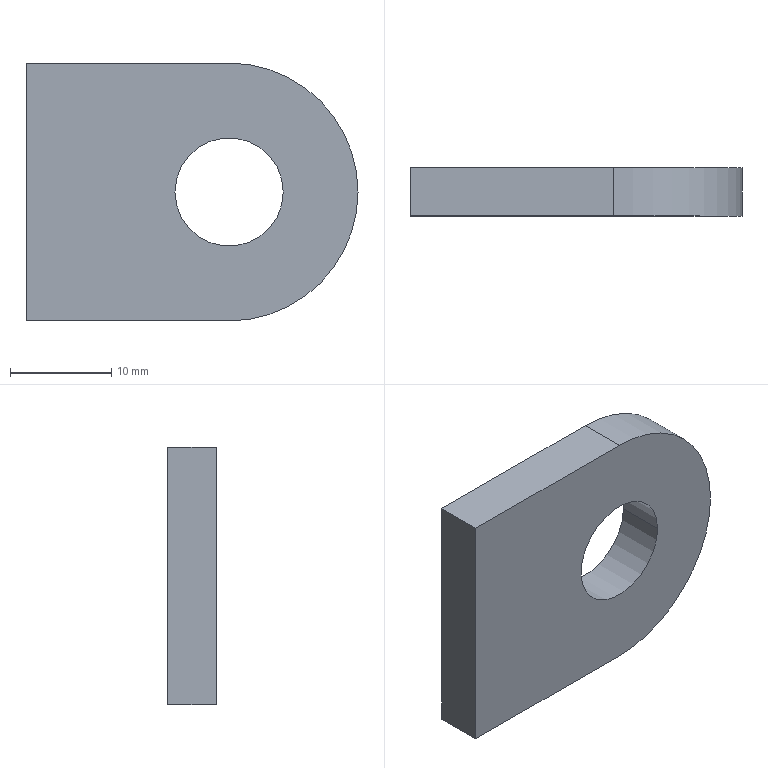Part | NX | features BREP 1 | 1 solid | 8 faces | box 32.715 x 4.763 x 25.4 mm | volume 3202 mm3 | plane 5 | cylinder 3 | commonest cylinder face diameters 10.668 x2 25.4 x1
STEP:
#1=CARTESIAN_POINT('',(0.,0.,12.7));
#2=VERTEX_POINT('',#1);
#3=CARTESIAN_POINT('',(20.015,0.,12.7));
#4=VERTEX_POINT('',#3);
#5=CARTESIAN_POINT('',(0.,0.,12.7));
#6=DIRECTION('',(1.,0.,0.));
#7=VECTOR('',#6,1000.);
#8=LINE('',#5,#7);
#9=EDGE_CURVE('',#2,#4,#8,.T.);
#10=ORIENTED_EDGE('',*,*,#9,.T.);
#11=CARTESIAN_POINT('',(20.015,0.,-12.7));
#12=VERTEX_POINT('',#11);
#13=CARTESIAN_POINT('',(20.015,0.,0.));
#14=DIRECTION('',(0.,1.,0.));
#15=DIRECTION('',(0.,0.,1.));
#16=AXIS2_PLACEMENT_3D('',#13,#14,#15);
#17=CIRCLE('',#16,12.7);
#18=EDGE_CURVE('',#4,#12,#17,.T.);
#19=ORIENTED_EDGE('',*,*,#18,.T.);
#20=CARTESIAN_POINT('',(0.,0.,-12.7));
#21=VERTEX_POINT('',#20);
#22=CARTESIAN_POINT('',(20.015,0.,-12.7));
#23=DIRECTION('',(-1.,0.,0.));
#24=VECTOR('',#23,1000.);
#25=LINE('',#22,#24);
#26=EDGE_CURVE('',#12,#21,#25,.T.);
#27=ORIENTED_EDGE('',*,*,#26,.T.);
#28=CARTESIAN_POINT('',(0.,0.,-12.7));
#29=DIRECTION('',(0.,0.,1.));
#30=VECTOR('',#29,1000.);
#31=LINE('',#28,#30);
#32=EDGE_CURVE('',#21,#2,#31,.T.);
#33=ORIENTED_EDGE('',*,*,#32,.T.);
#34=EDGE_LOOP('',(#10,#19,#27,#33));
#35=FACE_BOUND('',#34,.T.);
#36=CARTESIAN_POINT('',(25.349,0.,0.));
#37=VERTEX_POINT('',#36);
#38=CARTESIAN_POINT('',(14.681,0.,0.));
#39=VERTEX_POINT('',#38);
#40=CARTESIAN_POINT('',(20.015,0.,0.));
#41=DIRECTION('',(0.,1.,0.));
#42=DIRECTION('',(1.,0.,0.));
#43=AXIS2_PLACEMENT_3D('',#40,#41,#42);
#44=CIRCLE('',#43,5.334);
#45=EDGE_CURVE('',#37,#39,#44,.T.);
#46=ORIENTED_EDGE('',*,*,#45,.F.);
#47=CARTESIAN_POINT('',(20.015,0.,0.));
#48=DIRECTION('',(0.,1.,0.));
#49=DIRECTION('',(-1.,0.,0.));
#50=AXIS2_PLACEMENT_3D('',#47,#48,#49);
#51=CIRCLE('',#50,5.334);
#52=EDGE_CURVE('',#39,#37,#51,.T.);
#53=ORIENTED_EDGE('',*,*,#52,.F.);
#54=EDGE_LOOP('',(#46,#53));
#55=FACE_BOUND('',#54,.T.);
#56=CARTESIAN_POINT('',(0.,0.,0.));
#57=DIRECTION('',(0.,1.,0.));
#58=DIRECTION('',(1.,0.,0.));
#59=AXIS2_PLACEMENT_3D('',#56,#57,#58);
#60=PLANE('',#59);
#61=ADVANCED_FACE('',(#35,#55),#60,.T.);
#62=CARTESIAN_POINT('',(0.,-4.763,-12.7));
#63=VERTEX_POINT('',#62);
#64=CARTESIAN_POINT('',(0.,0.,-12.7));
#65=DIRECTION('',(0.,-1.,0.));
#66=VECTOR('',#65,1000.);
#67=LINE('',#64,#66);
#68=EDGE_CURVE('',#21,#63,#67,.T.);
#69=ORIENTED_EDGE('',*,*,#68,.T.);
#70=CARTESIAN_POINT('',(0.,-4.763,12.7));
#71=VERTEX_POINT('',#70);
#72=CARTESIAN_POINT('',(0.,-4.763,-12.7));
#73=DIRECTION('',(0.,0.,1.));
#74=VECTOR('',#73,1000.);
#75=LINE('',#72,#74);
#76=EDGE_CURVE('',#63,#71,#75,.T.);
#77=ORIENTED_EDGE('',*,*,#76,.T.);
#78=CARTESIAN_POINT('',(0.,0.,12.7));
#79=DIRECTION('',(0.,-1.,0.));
#80=VECTOR('',#79,1000.);
#81=LINE('',#78,#80);
#82=EDGE_CURVE('',#2,#71,#81,.T.);
#83=ORIENTED_EDGE('',*,*,#82,.F.);
#84=ORIENTED_EDGE('',*,*,#32,.F.);
#85=EDGE_LOOP('',(#69,#77,#83,#84));
#86=FACE_BOUND('',#85,.T.);
#87=CARTESIAN_POINT('',(0.,-2.381,0.));
#88=DIRECTION('',(-1.,0.,0.));
#89=DIRECTION('',(0.,0.,1.));
#90=AXIS2_PLACEMENT_3D('',#87,#88,#89);
#91=PLANE('',#90);
#92=ADVANCED_FACE('',(#86),#91,.T.);
#93=ORIENTED_EDGE('',*,*,#82,.T.);
#94=CARTESIAN_POINT('',(20.015,-4.763,12.7));
#95=VERTEX_POINT('',#94);
#96=CARTESIAN_POINT('',(0.,-4.763,12.7));
#97=DIRECTION('',(1.,0.,0.));
#98=VECTOR('',#97,1000.);
#99=LINE('',#96,#98);
#100=EDGE_CURVE('',#71,#95,#99,.T.);
#101=ORIENTED_EDGE('',*,*,#100,.T.);
#102=CARTESIAN_POINT('',(20.015,0.,12.7));
#103=DIRECTION('',(0.,-1.,0.));
#104=VECTOR('',#103,1000.);
#105=LINE('',#102,#104);
#106=EDGE_CURVE('',#4,#95,#105,.T.);
#107=ORIENTED_EDGE('',*,*,#106,.F.);
#108=ORIENTED_EDGE('',*,*,#9,.F.);
#109=EDGE_LOOP('',(#93,#101,#107,#108));
#110=FACE_BOUND('',#109,.T.);
#111=CARTESIAN_POINT('',(10.008,-2.381,12.7));
#112=DIRECTION('',(0.,0.,1.));
#113=DIRECTION('',(1.,0.,0.));
#114=AXIS2_PLACEMENT_3D('',#111,#112,#113);
#115=PLANE('',#114);
#116=ADVANCED_FACE('',(#110),#115,.T.);
#117=ORIENTED_EDGE('',*,*,#106,.T.);
#118=CARTESIAN_POINT('',(20.015,-4.763,-12.7));
#119=VERTEX_POINT('',#118);
#120=CARTESIAN_POINT('',(20.015,-4.763,0.));
#121=DIRECTION('',(0.,1.,0.));
#122=DIRECTION('',(0.,0.,1.));
#123=AXIS2_PLACEMENT_3D('',#120,#121,#122);
#124=CIRCLE('',#123,12.7);
#125=EDGE_CURVE('',#95,#119,#124,.T.);
#126=ORIENTED_EDGE('',*,*,#125,.T.);
#127=CARTESIAN_POINT('',(20.015,0.,-12.7));
#128=DIRECTION('',(0.,-1.,0.));
#129=VECTOR('',#128,1000.);
#130=LINE('',#127,#129);
#131=EDGE_CURVE('',#12,#119,#130,.T.);
#132=ORIENTED_EDGE('',*,*,#131,.F.);
#133=ORIENTED_EDGE('',*,*,#18,.F.);
#134=EDGE_LOOP('',(#117,#126,#132,#133));
#135=FACE_BOUND('',#134,.T.);
#136=CARTESIAN_POINT('',(20.015,-2.381,0.));
#137=DIRECTION('',(0.,1.,0.));
#138=DIRECTION('',(0.,0.,1.));
#139=AXIS2_PLACEMENT_3D('',#136,#137,#138);
#140=CYLINDRICAL_SURFACE('',#139,12.7);
#141=ADVANCED_FACE('',(#135),#140,.T.);
#142=ORIENTED_EDGE('',*,*,#131,.T.);
#143=CARTESIAN_POINT('',(20.015,-4.763,-12.7));
#144=DIRECTION('',(-1.,0.,0.));
#145=VECTOR('',#144,1000.);
#146=LINE('',#143,#145);
#147=EDGE_CURVE('',#119,#63,#146,.T.);
#148=ORIENTED_EDGE('',*,*,#147,.T.);
#149=ORIENTED_EDGE('',*,*,#68,.F.);
#150=ORIENTED_EDGE('',*,*,#26,.F.);
#151=EDGE_LOOP('',(#142,#148,#149,#150));
#152=FACE_BOUND('',#151,.T.);
#153=CARTESIAN_POINT('',(10.008,-2.381,-12.7));
#154=DIRECTION('',(0.,0.,-1.));
#155=DIRECTION('',(0.,-1.,0.));
#156=AXIS2_PLACEMENT_3D('',#153,#154,#155);
#157=PLANE('',#156);
#158=ADVANCED_FACE('',(#152),#157,.T.);
#159=ORIENTED_EDGE('',*,*,#147,.F.);
#160=ORIENTED_EDGE('',*,*,#125,.F.);
#161=ORIENTED_EDGE('',*,*,#100,.F.);
#162=ORIENTED_EDGE('',*,*,#76,.F.);
#163=EDGE_LOOP('',(#159,#160,#161,#162));
#164=FACE_BOUND('',#163,.T.);
#165=CARTESIAN_POINT('',(25.349,-4.763,0.));
#166=VERTEX_POINT('',#165);
#167=CARTESIAN_POINT('',(14.681,-4.763,0.));
#168=VERTEX_POINT('',#167);
#169=CARTESIAN_POINT('',(20.015,-4.763,0.));
#170=DIRECTION('',(0.,1.,0.));
#171=DIRECTION('',(1.,0.,0.));
#172=AXIS2_PLACEMENT_3D('',#169,#170,#171);
#173=CIRCLE('',#172,5.334);
#174=EDGE_CURVE('',#166,#168,#173,.T.);
#175=ORIENTED_EDGE('',*,*,#174,.T.);
#176=CARTESIAN_POINT('',(20.015,-4.763,0.));
#177=DIRECTION('',(0.,1.,0.));
#178=DIRECTION('',(-1.,0.,0.));
#179=AXIS2_PLACEMENT_3D('',#176,#177,#178);
#180=CIRCLE('',#179,5.334);
#181=EDGE_CURVE('',#168,#166,#180,.T.);
#182=ORIENTED_EDGE('',*,*,#181,.T.);
#183=EDGE_LOOP('',(#175,#182));
#184=FACE_BOUND('',#183,.T.);
#185=CARTESIAN_POINT('',(0.,-4.763,0.));
#186=DIRECTION('',(0.,1.,0.));
#187=DIRECTION('',(1.,0.,0.));
#188=AXIS2_PLACEMENT_3D('',#185,#186,#187);
#189=PLANE('',#188);
#190=ADVANCED_FACE('',(#164,#184),#189,.F.);
#191=CARTESIAN_POINT('',(25.349,0.,0.));
#192=DIRECTION('',(0.,-1.,0.));
#193=VECTOR('',#192,1000.);
#194=LINE('',#191,#193);
#195=EDGE_CURVE('',#166,#37,#194,.F.);
#196=ORIENTED_EDGE('',*,*,#195,.F.);
#197=ORIENTED_EDGE('',*,*,#181,.F.);
#198=CARTESIAN_POINT('',(14.681,0.,0.));
#199=DIRECTION('',(0.,-1.,0.));
#200=VECTOR('',#199,1000.);
#201=LINE('',#198,#200);
#202=EDGE_CURVE('',#168,#39,#201,.F.);
#203=ORIENTED_EDGE('',*,*,#202,.T.);
#204=ORIENTED_EDGE('',*,*,#52,.T.);
#205=EDGE_LOOP('',(#196,#197,#203,#204));
#206=FACE_BOUND('',#205,.T.);
#207=CARTESIAN_POINT('',(20.015,-2.381,0.));
#208=DIRECTION('',(0.,1.,0.));
#209=DIRECTION('',(-1.,0.,0.));
#210=AXIS2_PLACEMENT_3D('',#207,#208,#209);
#211=CYLINDRICAL_SURFACE('',#210,5.334);
#212=ADVANCED_FACE('',(#206),#211,.F.);
#213=ORIENTED_EDGE('',*,*,#202,.F.);
#214=ORIENTED_EDGE('',*,*,#174,.F.);
#215=ORIENTED_EDGE('',*,*,#195,.T.);
#216=ORIENTED_EDGE('',*,*,#45,.T.);
#217=EDGE_LOOP('',(#213,#214,#215,#216));
#218=FACE_BOUND('',#217,.T.);
#219=CARTESIAN_POINT('',(20.015,-2.381,0.));
#220=DIRECTION('',(0.,1.,0.));
#221=DIRECTION('',(1.,0.,0.));
#222=AXIS2_PLACEMENT_3D('',#219,#220,#221);
#223=CYLINDRICAL_SURFACE('',#222,5.334);
#224=ADVANCED_FACE('',(#218),#223,.F.);
#225=CLOSED_SHELL('',(#61,#92,#116,#141,#158,#190,#212,#224));
#226=MANIFOLD_SOLID_BREP('',#225);
#227=(LENGTH_UNIT()NAMED_UNIT(*)SI_UNIT(.MILLI.,.METRE.));
#228=UNCERTAINTY_MEASURE_WITH_UNIT(LENGTH_MEASURE(0.00001),#227,'','');
#229=(NAMED_UNIT(*)PLANE_ANGLE_UNIT()SI_UNIT($,.RADIAN.));
#230=(NAMED_UNIT(*)SI_UNIT($,.STERADIAN.)SOLID_ANGLE_UNIT());
#231=(GEOMETRIC_REPRESENTATION_CONTEXT(3)GLOBAL_UNCERTAINTY_ASSIGNED_CONTEXT((#228))GLOBAL_UNIT_ASSIGNED_CONTEXT((#227,#229,#230))REPRESENTATION_CONTEXT('',''));
#232=ADVANCED_BREP_SHAPE_REPRESENTATION('',(#226),#231);